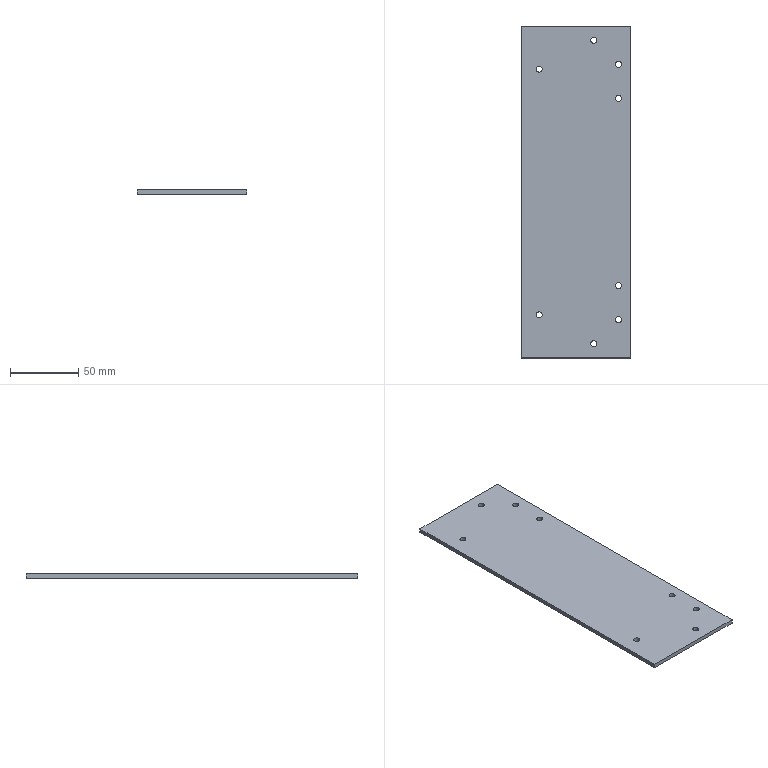Part | SolidWorks | features Cut 2, Extrusion 1, MirrorPattern 1 | 1 solid | 22 faces | box 80 x 243 x 3 mm | volume 57955 mm3 | cylinder 16 | plane 6 | commonest cylinder face diameters 4.4 x16
STEP:
#1=CARTESIAN_POINT('',(10.8,111.,3.));
#2=VERTEX_POINT('',#1);
#3=CARTESIAN_POINT('',(15.2,111.,3.));
#4=VERTEX_POINT('',#3);
#5=CARTESIAN_POINT('',(13.,111.,3.));
#6=DIRECTION('',(0.,0.,1.));
#7=DIRECTION('',(1.,0.,0.));
#8=AXIS2_PLACEMENT_3D('',#5,#6,#7);
#9=CIRCLE('',#8,2.2);
#10=EDGE_CURVE('',#2,#4,#9,.T.);
#11=ORIENTED_EDGE('',*,*,#10,.T.);
#12=CARTESIAN_POINT('',(15.2,111.,0.));
#13=VERTEX_POINT('',#12);
#14=CARTESIAN_POINT('',(15.2,111.,10.));
#15=DIRECTION('',(0.,0.,-1.));
#16=VECTOR('',#15,1000.);
#17=LINE('',#14,#16);
#18=EDGE_CURVE('',#4,#13,#17,.T.);
#19=ORIENTED_EDGE('',*,*,#18,.T.);
#20=CARTESIAN_POINT('',(10.8,111.,0.));
#21=VERTEX_POINT('',#20);
#22=CARTESIAN_POINT('',(13.,111.,0.));
#23=DIRECTION('',(0.,0.,-1.));
#24=DIRECTION('',(-1.,0.,0.));
#25=AXIS2_PLACEMENT_3D('',#22,#23,#24);
#26=CIRCLE('',#25,2.2);
#27=EDGE_CURVE('',#13,#21,#26,.T.);
#28=ORIENTED_EDGE('',*,*,#27,.T.);
#29=CARTESIAN_POINT('',(10.8,111.,10.));
#30=DIRECTION('',(0.,0.,-1.));
#31=VECTOR('',#30,1000.);
#32=LINE('',#29,#31);
#33=EDGE_CURVE('',#2,#21,#32,.T.);
#34=ORIENTED_EDGE('',*,*,#33,.F.);
#35=EDGE_LOOP('',(#11,#19,#28,#34));
#36=FACE_OUTER_BOUND('',#35,.T.);
#37=CARTESIAN_POINT('',(13.,111.,10.));
#38=DIRECTION('',(0.,0.,-1.));
#39=DIRECTION('',(-1.,0.,0.));
#40=AXIS2_PLACEMENT_3D('',#37,#38,#39);
#41=CYLINDRICAL_SURFACE('',#40,2.2);
#42=ADVANCED_FACE('',(#36),#41,.F.);
#43=CARTESIAN_POINT('',(-29.2,-90.,3.));
#44=VERTEX_POINT('',#43);
#45=CARTESIAN_POINT('',(-24.8,-90.,3.));
#46=VERTEX_POINT('',#45);
#47=CARTESIAN_POINT('',(-27.,-90.,3.));
#48=DIRECTION('',(0.,0.,1.));
#49=DIRECTION('',(1.,0.,0.));
#50=AXIS2_PLACEMENT_3D('',#47,#48,#49);
#51=CIRCLE('',#50,2.2);
#52=EDGE_CURVE('',#44,#46,#51,.T.);
#53=ORIENTED_EDGE('',*,*,#52,.T.);
#54=CARTESIAN_POINT('',(-24.8,-90.,0.));
#55=VERTEX_POINT('',#54);
#56=CARTESIAN_POINT('',(-24.8,-90.,10.));
#57=DIRECTION('',(0.,0.,-1.));
#58=VECTOR('',#57,1000.);
#59=LINE('',#56,#58);
#60=EDGE_CURVE('',#46,#55,#59,.T.);
#61=ORIENTED_EDGE('',*,*,#60,.T.);
#62=CARTESIAN_POINT('',(-29.2,-90.,0.));
#63=VERTEX_POINT('',#62);
#64=CARTESIAN_POINT('',(-27.,-90.,0.));
#65=DIRECTION('',(0.,0.,-1.));
#66=DIRECTION('',(-1.,0.,0.));
#67=AXIS2_PLACEMENT_3D('',#64,#65,#66);
#68=CIRCLE('',#67,2.2);
#69=EDGE_CURVE('',#55,#63,#68,.T.);
#70=ORIENTED_EDGE('',*,*,#69,.T.);
#71=CARTESIAN_POINT('',(-29.2,-90.,10.));
#72=DIRECTION('',(0.,0.,-1.));
#73=VECTOR('',#72,1000.);
#74=LINE('',#71,#73);
#75=EDGE_CURVE('',#44,#63,#74,.T.);
#76=ORIENTED_EDGE('',*,*,#75,.F.);
#77=EDGE_LOOP('',(#53,#61,#70,#76));
#78=FACE_OUTER_BOUND('',#77,.T.);
#79=CARTESIAN_POINT('',(-27.,-90.,10.));
#80=DIRECTION('',(0.,0.,-1.));
#81=DIRECTION('',(-1.,0.,0.));
#82=AXIS2_PLACEMENT_3D('',#79,#80,#81);
#83=CYLINDRICAL_SURFACE('',#82,2.2);
#84=ADVANCED_FACE('',(#78),#83,.F.);
#85=CARTESIAN_POINT('',(-29.2,90.,3.));
#86=VERTEX_POINT('',#85);
#87=CARTESIAN_POINT('',(-24.8,90.,3.));
#88=VERTEX_POINT('',#87);
#89=CARTESIAN_POINT('',(-27.,90.,3.));
#90=DIRECTION('',(0.,0.,1.));
#91=DIRECTION('',(1.,0.,0.));
#92=AXIS2_PLACEMENT_3D('',#89,#90,#91);
#93=CIRCLE('',#92,2.2);
#94=EDGE_CURVE('',#86,#88,#93,.T.);
#95=ORIENTED_EDGE('',*,*,#94,.T.);
#96=CARTESIAN_POINT('',(-24.8,90.,0.));
#97=VERTEX_POINT('',#96);
#98=CARTESIAN_POINT('',(-24.8,90.,10.));
#99=DIRECTION('',(0.,0.,-1.));
#100=VECTOR('',#99,1000.);
#101=LINE('',#98,#100);
#102=EDGE_CURVE('',#88,#97,#101,.T.);
#103=ORIENTED_EDGE('',*,*,#102,.T.);
#104=CARTESIAN_POINT('',(-29.2,90.,0.));
#105=VERTEX_POINT('',#104);
#106=CARTESIAN_POINT('',(-27.,90.,0.));
#107=DIRECTION('',(0.,0.,-1.));
#108=DIRECTION('',(-1.,0.,0.));
#109=AXIS2_PLACEMENT_3D('',#106,#107,#108);
#110=CIRCLE('',#109,2.2);
#111=EDGE_CURVE('',#97,#105,#110,.T.);
#112=ORIENTED_EDGE('',*,*,#111,.T.);
#113=CARTESIAN_POINT('',(-29.2,90.,10.));
#114=DIRECTION('',(0.,0.,-1.));
#115=VECTOR('',#114,1000.);
#116=LINE('',#113,#115);
#117=EDGE_CURVE('',#86,#105,#116,.T.);
#118=ORIENTED_EDGE('',*,*,#117,.F.);
#119=EDGE_LOOP('',(#95,#103,#112,#118));
#120=FACE_OUTER_BOUND('',#119,.T.);
#121=CARTESIAN_POINT('',(-27.,90.,10.));
#122=DIRECTION('',(0.,0.,-1.));
#123=DIRECTION('',(-1.,0.,0.));
#124=AXIS2_PLACEMENT_3D('',#121,#122,#123);
#125=CYLINDRICAL_SURFACE('',#124,2.2);
#126=ADVANCED_FACE('',(#120),#125,.F.);
#127=CARTESIAN_POINT('',(10.8,-111.,3.));
#128=VERTEX_POINT('',#127);
#129=CARTESIAN_POINT('',(15.2,-111.,3.));
#130=VERTEX_POINT('',#129);
#131=CARTESIAN_POINT('',(13.,-111.,3.));
#132=DIRECTION('',(0.,0.,1.));
#133=DIRECTION('',(1.,0.,0.));
#134=AXIS2_PLACEMENT_3D('',#131,#132,#133);
#135=CIRCLE('',#134,2.2);
#136=EDGE_CURVE('',#128,#130,#135,.T.);
#137=ORIENTED_EDGE('',*,*,#136,.T.);
#138=CARTESIAN_POINT('',(15.2,-111.,0.));
#139=VERTEX_POINT('',#138);
#140=CARTESIAN_POINT('',(15.2,-111.,10.));
#141=DIRECTION('',(0.,0.,-1.));
#142=VECTOR('',#141,1000.);
#143=LINE('',#140,#142);
#144=EDGE_CURVE('',#130,#139,#143,.T.);
#145=ORIENTED_EDGE('',*,*,#144,.T.);
#146=CARTESIAN_POINT('',(10.8,-111.,0.));
#147=VERTEX_POINT('',#146);
#148=CARTESIAN_POINT('',(13.,-111.,0.));
#149=DIRECTION('',(0.,0.,-1.));
#150=DIRECTION('',(-1.,0.,0.));
#151=AXIS2_PLACEMENT_3D('',#148,#149,#150);
#152=CIRCLE('',#151,2.2);
#153=EDGE_CURVE('',#139,#147,#152,.T.);
#154=ORIENTED_EDGE('',*,*,#153,.T.);
#155=CARTESIAN_POINT('',(10.8,-111.,10.));
#156=DIRECTION('',(0.,0.,-1.));
#157=VECTOR('',#156,1000.);
#158=LINE('',#155,#157);
#159=EDGE_CURVE('',#128,#147,#158,.T.);
#160=ORIENTED_EDGE('',*,*,#159,.F.);
#161=EDGE_LOOP('',(#137,#145,#154,#160));
#162=FACE_OUTER_BOUND('',#161,.T.);
#163=CARTESIAN_POINT('',(13.,-111.,10.));
#164=DIRECTION('',(0.,0.,-1.));
#165=DIRECTION('',(-1.,0.,0.));
#166=AXIS2_PLACEMENT_3D('',#163,#164,#165);
#167=CYLINDRICAL_SURFACE('',#166,2.2);
#168=ADVANCED_FACE('',(#162),#167,.F.);
#169=CARTESIAN_POINT('',(33.2,68.5,3.));
#170=VERTEX_POINT('',#169);
#171=CARTESIAN_POINT('',(28.8,68.5,3.));
#172=VERTEX_POINT('',#171);
#173=CARTESIAN_POINT('',(31.,68.5,3.));
#174=DIRECTION('',(0.,0.,-1.));
#175=DIRECTION('',(1.,0.,0.));
#176=AXIS2_PLACEMENT_3D('',#173,#174,#175);
#177=CIRCLE('',#176,2.2);
#178=EDGE_CURVE('',#170,#172,#177,.T.);
#179=ORIENTED_EDGE('',*,*,#178,.F.);
#180=CARTESIAN_POINT('',(33.2,68.5,0.));
#181=VERTEX_POINT('',#180);
#182=CARTESIAN_POINT('',(33.2,68.5,10.));
#183=DIRECTION('',(0.,0.,-1.));
#184=VECTOR('',#183,1000.);
#185=LINE('',#182,#184);
#186=EDGE_CURVE('',#170,#181,#185,.T.);
#187=ORIENTED_EDGE('',*,*,#186,.T.);
#188=CARTESIAN_POINT('',(28.8,68.5,0.));
#189=VERTEX_POINT('',#188);
#190=CARTESIAN_POINT('',(31.,68.5,0.));
#191=DIRECTION('',(0.,0.,1.));
#192=DIRECTION('',(-1.,0.,0.));
#193=AXIS2_PLACEMENT_3D('',#190,#191,#192);
#194=CIRCLE('',#193,2.2);
#195=EDGE_CURVE('',#189,#181,#194,.T.);
#196=ORIENTED_EDGE('',*,*,#195,.F.);
#197=CARTESIAN_POINT('',(28.8,68.5,10.));
#198=DIRECTION('',(0.,0.,-1.));
#199=VECTOR('',#198,1000.);
#200=LINE('',#197,#199);
#201=EDGE_CURVE('',#172,#189,#200,.T.);
#202=ORIENTED_EDGE('',*,*,#201,.F.);
#203=EDGE_LOOP('',(#179,#187,#196,#202));
#204=FACE_OUTER_BOUND('',#203,.T.);
#205=CARTESIAN_POINT('',(31.,68.5,10.));
#206=DIRECTION('',(0.,0.,-1.));
#207=DIRECTION('',(-1.,0.,0.));
#208=AXIS2_PLACEMENT_3D('',#205,#206,#207);
#209=CYLINDRICAL_SURFACE('',#208,2.2);
#210=ADVANCED_FACE('',(#204),#209,.F.);
#211=CARTESIAN_POINT('',(33.2,93.5,3.));
#212=VERTEX_POINT('',#211);
#213=CARTESIAN_POINT('',(28.8,93.5,3.));
#214=VERTEX_POINT('',#213);
#215=CARTESIAN_POINT('',(31.,93.5,3.));
#216=DIRECTION('',(0.,0.,-1.));
#217=DIRECTION('',(1.,0.,0.));
#218=AXIS2_PLACEMENT_3D('',#215,#216,#217);
#219=CIRCLE('',#218,2.2);
#220=EDGE_CURVE('',#212,#214,#219,.T.);
#221=ORIENTED_EDGE('',*,*,#220,.F.);
#222=CARTESIAN_POINT('',(33.2,93.5,0.));
#223=VERTEX_POINT('',#222);
#224=CARTESIAN_POINT('',(33.2,93.5,10.));
#225=DIRECTION('',(0.,0.,-1.));
#226=VECTOR('',#225,1000.);
#227=LINE('',#224,#226);
#228=EDGE_CURVE('',#212,#223,#227,.T.);
#229=ORIENTED_EDGE('',*,*,#228,.T.);
#230=CARTESIAN_POINT('',(28.8,93.5,0.));
#231=VERTEX_POINT('',#230);
#232=CARTESIAN_POINT('',(31.,93.5,0.));
#233=DIRECTION('',(0.,0.,1.));
#234=DIRECTION('',(-1.,0.,0.));
#235=AXIS2_PLACEMENT_3D('',#232,#233,#234);
#236=CIRCLE('',#235,2.2);
#237=EDGE_CURVE('',#231,#223,#236,.T.);
#238=ORIENTED_EDGE('',*,*,#237,.F.);
#239=CARTESIAN_POINT('',(28.8,93.5,10.));
#240=DIRECTION('',(0.,0.,-1.));
#241=VECTOR('',#240,1000.);
#242=LINE('',#239,#241);
#243=EDGE_CURVE('',#214,#231,#242,.T.);
#244=ORIENTED_EDGE('',*,*,#243,.F.);
#245=EDGE_LOOP('',(#221,#229,#238,#244));
#246=FACE_OUTER_BOUND('',#245,.T.);
#247=CARTESIAN_POINT('',(31.,93.5,10.));
#248=DIRECTION('',(0.,0.,-1.));
#249=DIRECTION('',(-1.,0.,0.));
#250=AXIS2_PLACEMENT_3D('',#247,#248,#249);
#251=CYLINDRICAL_SURFACE('',#250,2.2);
#252=ADVANCED_FACE('',(#246),#251,.F.);
#253=CARTESIAN_POINT('',(28.8,-68.5,3.));
#254=VERTEX_POINT('',#253);
#255=CARTESIAN_POINT('',(33.2,-68.5,3.));
#256=VERTEX_POINT('',#255);
#257=CARTESIAN_POINT('',(31.,-68.5,3.));
#258=DIRECTION('',(0.,0.,1.));
#259=DIRECTION('',(1.,0.,0.));
#260=AXIS2_PLACEMENT_3D('',#257,#258,#259);
#261=CIRCLE('',#260,2.2);
#262=EDGE_CURVE('',#254,#256,#261,.T.);
#263=ORIENTED_EDGE('',*,*,#262,.T.);
#264=CARTESIAN_POINT('',(33.2,-68.5,0.));
#265=VERTEX_POINT('',#264);
#266=CARTESIAN_POINT('',(33.2,-68.5,10.));
#267=DIRECTION('',(0.,0.,-1.));
#268=VECTOR('',#267,1000.);
#269=LINE('',#266,#268);
#270=EDGE_CURVE('',#256,#265,#269,.T.);
#271=ORIENTED_EDGE('',*,*,#270,.T.);
#272=CARTESIAN_POINT('',(28.8,-68.5,0.));
#273=VERTEX_POINT('',#272);
#274=CARTESIAN_POINT('',(31.,-68.5,0.));
#275=DIRECTION('',(0.,0.,-1.));
#276=DIRECTION('',(-1.,0.,0.));
#277=AXIS2_PLACEMENT_3D('',#274,#275,#276);
#278=CIRCLE('',#277,2.2);
#279=EDGE_CURVE('',#265,#273,#278,.T.);
#280=ORIENTED_EDGE('',*,*,#279,.T.);
#281=CARTESIAN_POINT('',(28.8,-68.5,10.));
#282=DIRECTION('',(0.,0.,-1.));
#283=VECTOR('',#282,1000.);
#284=LINE('',#281,#283);
#285=EDGE_CURVE('',#254,#273,#284,.T.);
#286=ORIENTED_EDGE('',*,*,#285,.F.);
#287=EDGE_LOOP('',(#263,#271,#280,#286));
#288=FACE_OUTER_BOUND('',#287,.T.);
#289=CARTESIAN_POINT('',(31.,-68.5,10.));
#290=DIRECTION('',(0.,0.,-1.));
#291=DIRECTION('',(-1.,0.,0.));
#292=AXIS2_PLACEMENT_3D('',#289,#290,#291);
#293=CYLINDRICAL_SURFACE('',#292,2.2);
#294=ADVANCED_FACE('',(#288),#293,.F.);
#295=CARTESIAN_POINT('',(28.8,-93.5,3.));
#296=VERTEX_POINT('',#295);
#297=CARTESIAN_POINT('',(33.2,-93.5,3.));
#298=VERTEX_POINT('',#297);
#299=CARTESIAN_POINT('',(31.,-93.5,3.));
#300=DIRECTION('',(0.,0.,1.));
#301=DIRECTION('',(1.,0.,0.));
#302=AXIS2_PLACEMENT_3D('',#299,#300,#301);
#303=CIRCLE('',#302,2.2);
#304=EDGE_CURVE('',#296,#298,#303,.T.);
#305=ORIENTED_EDGE('',*,*,#304,.T.);
#306=CARTESIAN_POINT('',(33.2,-93.5,0.));
#307=VERTEX_POINT('',#306);
#308=CARTESIAN_POINT('',(33.2,-93.5,10.));
#309=DIRECTION('',(0.,0.,-1.));
#310=VECTOR('',#309,1000.);
#311=LINE('',#308,#310);
#312=EDGE_CURVE('',#298,#307,#311,.T.);
#313=ORIENTED_EDGE('',*,*,#312,.T.);
#314=CARTESIAN_POINT('',(28.8,-93.5,0.));
#315=VERTEX_POINT('',#314);
#316=CARTESIAN_POINT('',(31.,-93.5,0.));
#317=DIRECTION('',(0.,0.,-1.));
#318=DIRECTION('',(-1.,0.,0.));
#319=AXIS2_PLACEMENT_3D('',#316,#317,#318);
#320=CIRCLE('',#319,2.2);
#321=EDGE_CURVE('',#307,#315,#320,.T.);
#322=ORIENTED_EDGE('',*,*,#321,.T.);
#323=CARTESIAN_POINT('',(28.8,-93.5,10.));
#324=DIRECTION('',(0.,0.,-1.));
#325=VECTOR('',#324,1000.);
#326=LINE('',#323,#325);
#327=EDGE_CURVE('',#296,#315,#326,.T.);
#328=ORIENTED_EDGE('',*,*,#327,.F.);
#329=EDGE_LOOP('',(#305,#313,#322,#328));
#330=FACE_OUTER_BOUND('',#329,.T.);
#331=CARTESIAN_POINT('',(31.,-93.5,10.));
#332=DIRECTION('',(0.,0.,-1.));
#333=DIRECTION('',(-1.,0.,0.));
#334=AXIS2_PLACEMENT_3D('',#331,#332,#333);
#335=CYLINDRICAL_SURFACE('',#334,2.2);
#336=ADVANCED_FACE('',(#330),#335,.F.);
#337=CARTESIAN_POINT('',(-40.,121.5,0.));
#338=VERTEX_POINT('',#337);
#339=CARTESIAN_POINT('',(-40.,-121.5,0.));
#340=VERTEX_POINT('',#339);
#341=CARTESIAN_POINT('',(-40.,-121.5,0.));
#342=DIRECTION('',(0.,-1.,0.));
#343=VECTOR('',#342,1000.);
#344=LINE('',#341,#343);
#345=EDGE_CURVE('',#338,#340,#344,.T.);
#346=ORIENTED_EDGE('',*,*,#345,.T.);
#347=CARTESIAN_POINT('',(-40.,-121.5,3.));
#348=VERTEX_POINT('',#347);
#349=CARTESIAN_POINT('',(-40.,-121.5,3.));
#350=DIRECTION('',(0.,0.,-1.));
#351=VECTOR('',#350,1000.);
#352=LINE('',#349,#351);
#353=EDGE_CURVE('',#348,#340,#352,.T.);
#354=ORIENTED_EDGE('',*,*,#353,.F.);
#355=CARTESIAN_POINT('',(-40.,121.5,3.));
#356=VERTEX_POINT('',#355);
#357=CARTESIAN_POINT('',(-40.,-121.5,3.));
#358=DIRECTION('',(0.,-1.,0.));
#359=VECTOR('',#358,1000.);
#360=LINE('',#357,#359);
#361=EDGE_CURVE('',#356,#348,#360,.T.);
#362=ORIENTED_EDGE('',*,*,#361,.F.);
#363=CARTESIAN_POINT('',(-40.,121.5,3.));
#364=DIRECTION('',(0.,0.,-1.));
#365=VECTOR('',#364,1000.);
#366=LINE('',#363,#365);
#367=EDGE_CURVE('',#356,#338,#366,.T.);
#368=ORIENTED_EDGE('',*,*,#367,.T.);
#369=EDGE_LOOP('',(#346,#354,#362,#368));
#370=FACE_OUTER_BOUND('',#369,.T.);
#371=CARTESIAN_POINT('',(-40.,-121.5,3.));
#372=DIRECTION('',(1.,0.,0.));
#373=DIRECTION('',(0.,0.,-1.));
#374=AXIS2_PLACEMENT_3D('',#371,#372,#373);
#375=PLANE('',#374);
#376=ADVANCED_FACE('',(#370),#375,.F.);
#377=CARTESIAN_POINT('',(40.,-121.5,0.));
#378=VERTEX_POINT('',#377);
#379=CARTESIAN_POINT('',(40.,-121.5,0.));
#380=DIRECTION('',(1.,0.,0.));
#381=VECTOR('',#380,1000.);
#382=LINE('',#379,#381);
#383=EDGE_CURVE('',#340,#378,#382,.T.);
#384=ORIENTED_EDGE('',*,*,#383,.T.);
#385=CARTESIAN_POINT('',(40.,-121.5,3.));
#386=VERTEX_POINT('',#385);
#387=CARTESIAN_POINT('',(40.,-121.5,3.));
#388=DIRECTION('',(0.,0.,-1.));
#389=VECTOR('',#388,1000.);
#390=LINE('',#387,#389);
#391=EDGE_CURVE('',#386,#378,#390,.T.);
#392=ORIENTED_EDGE('',*,*,#391,.F.);
#393=CARTESIAN_POINT('',(40.,-121.5,3.));
#394=DIRECTION('',(1.,0.,0.));
#395=VECTOR('',#394,1000.);
#396=LINE('',#393,#395);
#397=EDGE_CURVE('',#348,#386,#396,.T.);
#398=ORIENTED_EDGE('',*,*,#397,.F.);
#399=ORIENTED_EDGE('',*,*,#353,.T.);
#400=EDGE_LOOP('',(#384,#392,#398,#399));
#401=FACE_OUTER_BOUND('',#400,.T.);
#402=CARTESIAN_POINT('',(40.,-121.5,3.));
#403=DIRECTION('',(0.,1.,0.));
#404=DIRECTION('',(-1.,0.,0.));
#405=AXIS2_PLACEMENT_3D('',#402,#403,#404);
#406=PLANE('',#405);
#407=ADVANCED_FACE('',(#401),#406,.F.);
#408=CARTESIAN_POINT('',(40.,121.5,0.));
#409=VERTEX_POINT('',#408);
#410=CARTESIAN_POINT('',(40.,-121.5,0.));
#411=DIRECTION('',(0.,1.,0.));
#412=VECTOR('',#411,1000.);
#413=LINE('',#410,#412);
#414=EDGE_CURVE('',#378,#409,#413,.T.);
#415=ORIENTED_EDGE('',*,*,#414,.T.);
#416=CARTESIAN_POINT('',(40.,121.5,3.));
#417=VERTEX_POINT('',#416);
#418=CARTESIAN_POINT('',(40.,121.5,3.));
#419=DIRECTION('',(0.,0.,-1.));
#420=VECTOR('',#419,1000.);
#421=LINE('',#418,#420);
#422=EDGE_CURVE('',#417,#409,#421,.T.);
#423=ORIENTED_EDGE('',*,*,#422,.F.);
#424=CARTESIAN_POINT('',(40.,-121.5,3.));
#425=DIRECTION('',(0.,1.,0.));
#426=VECTOR('',#425,1000.);
#427=LINE('',#424,#426);
#428=EDGE_CURVE('',#386,#417,#427,.T.);
#429=ORIENTED_EDGE('',*,*,#428,.F.);
#430=ORIENTED_EDGE('',*,*,#391,.T.);
#431=EDGE_LOOP('',(#415,#423,#429,#430));
#432=FACE_OUTER_BOUND('',#431,.T.);
#433=CARTESIAN_POINT('',(40.,-121.5,3.));
#434=DIRECTION('',(-1.,0.,0.));
#435=DIRECTION('',(0.,0.,1.));
#436=AXIS2_PLACEMENT_3D('',#433,#434,#435);
#437=PLANE('',#436);
#438=ADVANCED_FACE('',(#432),#437,.F.);
#439=CARTESIAN_POINT('',(40.,121.5,0.));
#440=DIRECTION('',(-1.,0.,0.));
#441=VECTOR('',#440,1000.);
#442=LINE('',#439,#441);
#443=EDGE_CURVE('',#409,#338,#442,.T.);
#444=ORIENTED_EDGE('',*,*,#443,.T.);
#445=ORIENTED_EDGE('',*,*,#367,.F.);
#446=CARTESIAN_POINT('',(40.,121.5,3.));
#447=DIRECTION('',(-1.,0.,0.));
#448=VECTOR('',#447,1000.);
#449=LINE('',#446,#448);
#450=EDGE_CURVE('',#417,#356,#449,.T.);
#451=ORIENTED_EDGE('',*,*,#450,.F.);
#452=ORIENTED_EDGE('',*,*,#422,.T.);
#453=EDGE_LOOP('',(#444,#445,#451,#452));
#454=FACE_OUTER_BOUND('',#453,.T.);
#455=CARTESIAN_POINT('',(40.,121.5,3.));
#456=DIRECTION('',(0.,-1.,0.));
#457=DIRECTION('',(1.,0.,0.));
#458=AXIS2_PLACEMENT_3D('',#455,#456,#457);
#459=PLANE('',#458);
#460=ADVANCED_FACE('',(#454),#459,.F.);
#461=ORIENTED_EDGE('',*,*,#10,.F.);
#462=CARTESIAN_POINT('',(13.,111.,3.));
#463=DIRECTION('',(0.,0.,1.));
#464=DIRECTION('',(1.,0.,0.));
#465=AXIS2_PLACEMENT_3D('',#462,#463,#464);
#466=CIRCLE('',#465,2.2);
#467=EDGE_CURVE('',#4,#2,#466,.T.);
#468=ORIENTED_EDGE('',*,*,#467,.F.);
#469=EDGE_LOOP('',(#461,#468));
#470=FACE_BOUND('',#469,.T.);
#471=ORIENTED_EDGE('',*,*,#52,.F.);
#472=CARTESIAN_POINT('',(-27.,-90.,3.));
#473=DIRECTION('',(0.,0.,1.));
#474=DIRECTION('',(1.,0.,0.));
#475=AXIS2_PLACEMENT_3D('',#472,#473,#474);
#476=CIRCLE('',#475,2.2);
#477=EDGE_CURVE('',#46,#44,#476,.T.);
#478=ORIENTED_EDGE('',*,*,#477,.F.);
#479=EDGE_LOOP('',(#471,#478));
#480=FACE_BOUND('',#479,.T.);
#481=ORIENTED_EDGE('',*,*,#94,.F.);
#482=CARTESIAN_POINT('',(-27.,90.,3.));
#483=DIRECTION('',(0.,0.,1.));
#484=DIRECTION('',(1.,0.,0.));
#485=AXIS2_PLACEMENT_3D('',#482,#483,#484);
#486=CIRCLE('',#485,2.2);
#487=EDGE_CURVE('',#88,#86,#486,.T.);
#488=ORIENTED_EDGE('',*,*,#487,.F.);
#489=EDGE_LOOP('',(#481,#488));
#490=FACE_BOUND('',#489,.T.);
#491=ORIENTED_EDGE('',*,*,#136,.F.);
#492=CARTESIAN_POINT('',(13.,-111.,3.));
#493=DIRECTION('',(0.,0.,1.));
#494=DIRECTION('',(1.,0.,0.));
#495=AXIS2_PLACEMENT_3D('',#492,#493,#494);
#496=CIRCLE('',#495,2.2);
#497=EDGE_CURVE('',#130,#128,#496,.T.);
#498=ORIENTED_EDGE('',*,*,#497,.F.);
#499=EDGE_LOOP('',(#491,#498));
#500=FACE_BOUND('',#499,.T.);
#501=CARTESIAN_POINT('',(31.,68.5,3.));
#502=DIRECTION('',(0.,0.,-1.));
#503=DIRECTION('',(1.,0.,0.));
#504=AXIS2_PLACEMENT_3D('',#501,#502,#503);
#505=CIRCLE('',#504,2.2);
#506=EDGE_CURVE('',#172,#170,#505,.T.);
#507=ORIENTED_EDGE('',*,*,#506,.T.);
#508=ORIENTED_EDGE('',*,*,#178,.T.);
#509=EDGE_LOOP('',(#507,#508));
#510=FACE_BOUND('',#509,.T.);
#511=CARTESIAN_POINT('',(31.,93.5,3.));
#512=DIRECTION('',(0.,0.,-1.));
#513=DIRECTION('',(1.,0.,0.));
#514=AXIS2_PLACEMENT_3D('',#511,#512,#513);
#515=CIRCLE('',#514,2.2);
#516=EDGE_CURVE('',#214,#212,#515,.T.);
#517=ORIENTED_EDGE('',*,*,#516,.T.);
#518=ORIENTED_EDGE('',*,*,#220,.T.);
#519=EDGE_LOOP('',(#517,#518));
#520=FACE_BOUND('',#519,.T.);
#521=ORIENTED_EDGE('',*,*,#262,.F.);
#522=CARTESIAN_POINT('',(31.,-68.5,3.));
#523=DIRECTION('',(0.,0.,1.));
#524=DIRECTION('',(1.,0.,0.));
#525=AXIS2_PLACEMENT_3D('',#522,#523,#524);
#526=CIRCLE('',#525,2.2);
#527=EDGE_CURVE('',#256,#254,#526,.T.);
#528=ORIENTED_EDGE('',*,*,#527,.F.);
#529=EDGE_LOOP('',(#521,#528));
#530=FACE_BOUND('',#529,.T.);
#531=ORIENTED_EDGE('',*,*,#304,.F.);
#532=CARTESIAN_POINT('',(31.,-93.5,3.));
#533=DIRECTION('',(0.,0.,1.));
#534=DIRECTION('',(1.,0.,0.));
#535=AXIS2_PLACEMENT_3D('',#532,#533,#534);
#536=CIRCLE('',#535,2.2);
#537=EDGE_CURVE('',#298,#296,#536,.T.);
#538=ORIENTED_EDGE('',*,*,#537,.F.);
#539=EDGE_LOOP('',(#531,#538));
#540=FACE_BOUND('',#539,.T.);
#541=ORIENTED_EDGE('',*,*,#361,.T.);
#542=ORIENTED_EDGE('',*,*,#397,.T.);
#543=ORIENTED_EDGE('',*,*,#428,.T.);
#544=ORIENTED_EDGE('',*,*,#450,.T.);
#545=EDGE_LOOP('',(#541,#542,#543,#544));
#546=FACE_OUTER_BOUND('',#545,.T.);
#547=CARTESIAN_POINT('',(0.,0.,3.));
#548=DIRECTION('',(0.,0.,1.));
#549=DIRECTION('',(1.,0.,0.));
#550=AXIS2_PLACEMENT_3D('',#547,#548,#549);
#551=PLANE('',#550);
#552=ADVANCED_FACE('',(#470,#480,#490,#500,#510,#520,#530,#540,#546),#551,.T.);
#553=CARTESIAN_POINT('',(13.,111.,0.));
#554=DIRECTION('',(0.,0.,-1.));
#555=DIRECTION('',(-1.,0.,0.));
#556=AXIS2_PLACEMENT_3D('',#553,#554,#555);
#557=CIRCLE('',#556,2.2);
#558=EDGE_CURVE('',#21,#13,#557,.T.);
#559=ORIENTED_EDGE('',*,*,#558,.F.);
#560=ORIENTED_EDGE('',*,*,#27,.F.);
#561=EDGE_LOOP('',(#559,#560));
#562=FACE_BOUND('',#561,.T.);
#563=CARTESIAN_POINT('',(-27.,-90.,0.));
#564=DIRECTION('',(0.,0.,-1.));
#565=DIRECTION('',(-1.,0.,0.));
#566=AXIS2_PLACEMENT_3D('',#563,#564,#565);
#567=CIRCLE('',#566,2.2);
#568=EDGE_CURVE('',#63,#55,#567,.T.);
#569=ORIENTED_EDGE('',*,*,#568,.F.);
#570=ORIENTED_EDGE('',*,*,#69,.F.);
#571=EDGE_LOOP('',(#569,#570));
#572=FACE_BOUND('',#571,.T.);
#573=CARTESIAN_POINT('',(-27.,90.,0.));
#574=DIRECTION('',(0.,0.,-1.));
#575=DIRECTION('',(-1.,0.,0.));
#576=AXIS2_PLACEMENT_3D('',#573,#574,#575);
#577=CIRCLE('',#576,2.2);
#578=EDGE_CURVE('',#105,#97,#577,.T.);
#579=ORIENTED_EDGE('',*,*,#578,.F.);
#580=ORIENTED_EDGE('',*,*,#111,.F.);
#581=EDGE_LOOP('',(#579,#580));
#582=FACE_BOUND('',#581,.T.);
#583=CARTESIAN_POINT('',(13.,-111.,0.));
#584=DIRECTION('',(0.,0.,-1.));
#585=DIRECTION('',(-1.,0.,0.));
#586=AXIS2_PLACEMENT_3D('',#583,#584,#585);
#587=CIRCLE('',#586,2.2);
#588=EDGE_CURVE('',#147,#139,#587,.T.);
#589=ORIENTED_EDGE('',*,*,#588,.F.);
#590=ORIENTED_EDGE('',*,*,#153,.F.);
#591=EDGE_LOOP('',(#589,#590));
#592=FACE_BOUND('',#591,.T.);
#593=ORIENTED_EDGE('',*,*,#195,.T.);
#594=CARTESIAN_POINT('',(31.,68.5,0.));
#595=DIRECTION('',(0.,0.,1.));
#596=DIRECTION('',(-1.,0.,0.));
#597=AXIS2_PLACEMENT_3D('',#594,#595,#596);
#598=CIRCLE('',#597,2.2);
#599=EDGE_CURVE('',#181,#189,#598,.T.);
#600=ORIENTED_EDGE('',*,*,#599,.T.);
#601=EDGE_LOOP('',(#593,#600));
#602=FACE_BOUND('',#601,.T.);
#603=ORIENTED_EDGE('',*,*,#237,.T.);
#604=CARTESIAN_POINT('',(31.,93.5,0.));
#605=DIRECTION('',(0.,0.,1.));
#606=DIRECTION('',(-1.,0.,0.));
#607=AXIS2_PLACEMENT_3D('',#604,#605,#606);
#608=CIRCLE('',#607,2.2);
#609=EDGE_CURVE('',#223,#231,#608,.T.);
#610=ORIENTED_EDGE('',*,*,#609,.T.);
#611=EDGE_LOOP('',(#603,#610));
#612=FACE_BOUND('',#611,.T.);
#613=CARTESIAN_POINT('',(31.,-68.5,0.));
#614=DIRECTION('',(0.,0.,-1.));
#615=DIRECTION('',(-1.,0.,0.));
#616=AXIS2_PLACEMENT_3D('',#613,#614,#615);
#617=CIRCLE('',#616,2.2);
#618=EDGE_CURVE('',#273,#265,#617,.T.);
#619=ORIENTED_EDGE('',*,*,#618,.F.);
#620=ORIENTED_EDGE('',*,*,#279,.F.);
#621=EDGE_LOOP('',(#619,#620));
#622=FACE_BOUND('',#621,.T.);
#623=CARTESIAN_POINT('',(31.,-93.5,0.));
#624=DIRECTION('',(0.,0.,-1.));
#625=DIRECTION('',(-1.,0.,0.));
#626=AXIS2_PLACEMENT_3D('',#623,#624,#625);
#627=CIRCLE('',#626,2.2);
#628=EDGE_CURVE('',#315,#307,#627,.T.);
#629=ORIENTED_EDGE('',*,*,#628,.F.);
#630=ORIENTED_EDGE('',*,*,#321,.F.);
#631=EDGE_LOOP('',(#629,#630));
#632=FACE_BOUND('',#631,.T.);
#633=ORIENTED_EDGE('',*,*,#345,.F.);
#634=ORIENTED_EDGE('',*,*,#443,.F.);
#635=ORIENTED_EDGE('',*,*,#414,.F.);
#636=ORIENTED_EDGE('',*,*,#383,.F.);
#637=EDGE_LOOP('',(#633,#634,#635,#636));
#638=FACE_OUTER_BOUND('',#637,.T.);
#639=CARTESIAN_POINT('',(0.,0.,0.));
#640=DIRECTION('',(0.,0.,1.));
#641=DIRECTION('',(1.,0.,0.));
#642=AXIS2_PLACEMENT_3D('',#639,#640,#641);
#643=PLANE('',#642);
#644=ADVANCED_FACE('',(#562,#572,#582,#592,#602,#612,#622,#632,#638),#643,.F.);
#645=ORIENTED_EDGE('',*,*,#312,.F.);
#646=ORIENTED_EDGE('',*,*,#537,.T.);
#647=ORIENTED_EDGE('',*,*,#327,.T.);
#648=ORIENTED_EDGE('',*,*,#628,.T.);
#649=EDGE_LOOP('',(#645,#646,#647,#648));
#650=FACE_OUTER_BOUND('',#649,.T.);
#651=CARTESIAN_POINT('',(31.,-93.5,10.));
#652=DIRECTION('',(0.,0.,-1.));
#653=DIRECTION('',(-1.,0.,0.));
#654=AXIS2_PLACEMENT_3D('',#651,#652,#653);
#655=CYLINDRICAL_SURFACE('',#654,2.2);
#656=ADVANCED_FACE('',(#650),#655,.F.);
#657=ORIENTED_EDGE('',*,*,#270,.F.);
#658=ORIENTED_EDGE('',*,*,#527,.T.);
#659=ORIENTED_EDGE('',*,*,#285,.T.);
#660=ORIENTED_EDGE('',*,*,#618,.T.);
#661=EDGE_LOOP('',(#657,#658,#659,#660));
#662=FACE_OUTER_BOUND('',#661,.T.);
#663=CARTESIAN_POINT('',(31.,-68.5,10.));
#664=DIRECTION('',(0.,0.,-1.));
#665=DIRECTION('',(-1.,0.,0.));
#666=AXIS2_PLACEMENT_3D('',#663,#664,#665);
#667=CYLINDRICAL_SURFACE('',#666,2.2);
#668=ADVANCED_FACE('',(#662),#667,.F.);
#669=ORIENTED_EDGE('',*,*,#228,.F.);
#670=ORIENTED_EDGE('',*,*,#516,.F.);
#671=ORIENTED_EDGE('',*,*,#243,.T.);
#672=ORIENTED_EDGE('',*,*,#609,.F.);
#673=EDGE_LOOP('',(#669,#670,#671,#672));
#674=FACE_OUTER_BOUND('',#673,.T.);
#675=CARTESIAN_POINT('',(31.,93.5,10.));
#676=DIRECTION('',(0.,0.,-1.));
#677=DIRECTION('',(-1.,0.,0.));
#678=AXIS2_PLACEMENT_3D('',#675,#676,#677);
#679=CYLINDRICAL_SURFACE('',#678,2.2);
#680=ADVANCED_FACE('',(#674),#679,.F.);
#681=ORIENTED_EDGE('',*,*,#186,.F.);
#682=ORIENTED_EDGE('',*,*,#506,.F.);
#683=ORIENTED_EDGE('',*,*,#201,.T.);
#684=ORIENTED_EDGE('',*,*,#599,.F.);
#685=EDGE_LOOP('',(#681,#682,#683,#684));
#686=FACE_OUTER_BOUND('',#685,.T.);
#687=CARTESIAN_POINT('',(31.,68.5,10.));
#688=DIRECTION('',(0.,0.,-1.));
#689=DIRECTION('',(-1.,0.,0.));
#690=AXIS2_PLACEMENT_3D('',#687,#688,#689);
#691=CYLINDRICAL_SURFACE('',#690,2.2);
#692=ADVANCED_FACE('',(#686),#691,.F.);
#693=ORIENTED_EDGE('',*,*,#144,.F.);
#694=ORIENTED_EDGE('',*,*,#497,.T.);
#695=ORIENTED_EDGE('',*,*,#159,.T.);
#696=ORIENTED_EDGE('',*,*,#588,.T.);
#697=EDGE_LOOP('',(#693,#694,#695,#696));
#698=FACE_OUTER_BOUND('',#697,.T.);
#699=CARTESIAN_POINT('',(13.,-111.,10.));
#700=DIRECTION('',(0.,0.,-1.));
#701=DIRECTION('',(-1.,0.,0.));
#702=AXIS2_PLACEMENT_3D('',#699,#700,#701);
#703=CYLINDRICAL_SURFACE('',#702,2.2);
#704=ADVANCED_FACE('',(#698),#703,.F.);
#705=ORIENTED_EDGE('',*,*,#102,.F.);
#706=ORIENTED_EDGE('',*,*,#487,.T.);
#707=ORIENTED_EDGE('',*,*,#117,.T.);
#708=ORIENTED_EDGE('',*,*,#578,.T.);
#709=EDGE_LOOP('',(#705,#706,#707,#708));
#710=FACE_OUTER_BOUND('',#709,.T.);
#711=CARTESIAN_POINT('',(-27.,90.,10.));
#712=DIRECTION('',(0.,0.,-1.));
#713=DIRECTION('',(-1.,0.,0.));
#714=AXIS2_PLACEMENT_3D('',#711,#712,#713);
#715=CYLINDRICAL_SURFACE('',#714,2.2);
#716=ADVANCED_FACE('',(#710),#715,.F.);
#717=ORIENTED_EDGE('',*,*,#60,.F.);
#718=ORIENTED_EDGE('',*,*,#477,.T.);
#719=ORIENTED_EDGE('',*,*,#75,.T.);
#720=ORIENTED_EDGE('',*,*,#568,.T.);
#721=EDGE_LOOP('',(#717,#718,#719,#720));
#722=FACE_OUTER_BOUND('',#721,.T.);
#723=CARTESIAN_POINT('',(-27.,-90.,10.));
#724=DIRECTION('',(0.,0.,-1.));
#725=DIRECTION('',(-1.,0.,0.));
#726=AXIS2_PLACEMENT_3D('',#723,#724,#725);
#727=CYLINDRICAL_SURFACE('',#726,2.2);
#728=ADVANCED_FACE('',(#722),#727,.F.);
#729=ORIENTED_EDGE('',*,*,#18,.F.);
#730=ORIENTED_EDGE('',*,*,#467,.T.);
#731=ORIENTED_EDGE('',*,*,#33,.T.);
#732=ORIENTED_EDGE('',*,*,#558,.T.);
#733=EDGE_LOOP('',(#729,#730,#731,#732));
#734=FACE_OUTER_BOUND('',#733,.T.);
#735=CARTESIAN_POINT('',(13.,111.,10.));
#736=DIRECTION('',(0.,0.,-1.));
#737=DIRECTION('',(-1.,0.,0.));
#738=AXIS2_PLACEMENT_3D('',#735,#736,#737);
#739=CYLINDRICAL_SURFACE('',#738,2.2);
#740=ADVANCED_FACE('',(#734),#739,.F.);
#741=CLOSED_SHELL('',(#42,#84,#126,#168,#210,#252,#294,#336,#376,#407,#438,#460,#552,#644,#656,#668,#680,#692,#704,#716,#728,#740));
#742=MANIFOLD_SOLID_BREP('',#741);
#743=CARTESIAN_POINT('',(0.,0.,0.));
#744=DIRECTION('',(0.,0.,1.));
#745=DIRECTION('',(1.,0.,0.));
#746=AXIS2_PLACEMENT_3D('',#743,#744,#745);
#747=(LENGTH_UNIT()NAMED_UNIT(*)SI_UNIT(.MILLI.,.METRE.));
#748=UNCERTAINTY_MEASURE_WITH_UNIT(LENGTH_MEASURE(0.00001),#747,'','');
#749=(NAMED_UNIT(*)PLANE_ANGLE_UNIT()SI_UNIT($,.RADIAN.));
#750=(NAMED_UNIT(*)SI_UNIT($,.STERADIAN.)SOLID_ANGLE_UNIT());
#751=(GEOMETRIC_REPRESENTATION_CONTEXT(3)GLOBAL_UNCERTAINTY_ASSIGNED_CONTEXT((#748))GLOBAL_UNIT_ASSIGNED_CONTEXT((#747,#749,#750))REPRESENTATION_CONTEXT('',''));
#752=ADVANCED_BREP_SHAPE_REPRESENTATION('',(#742,#746),#751);